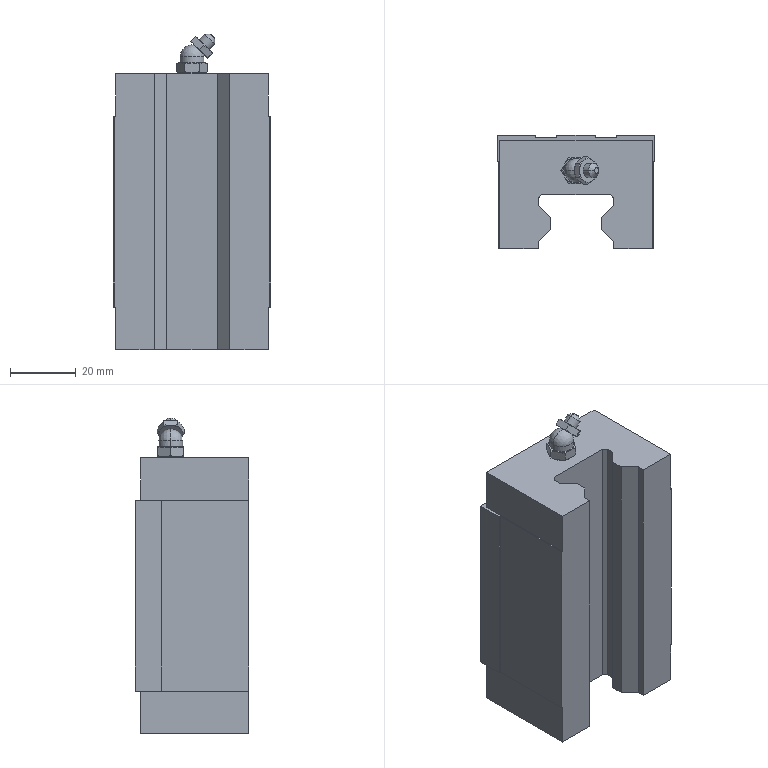Part | SolidWorks | features BaseBody 1 | 1 solid | 107 faces | box 48 x 34.5 x 96 mm | volume 106215 mm3 | plane 61 | cone 30 | cylinder 14 | sphere 2 | commonest cylinder face diameters 6 x8 7.2 x4 4.32 x2